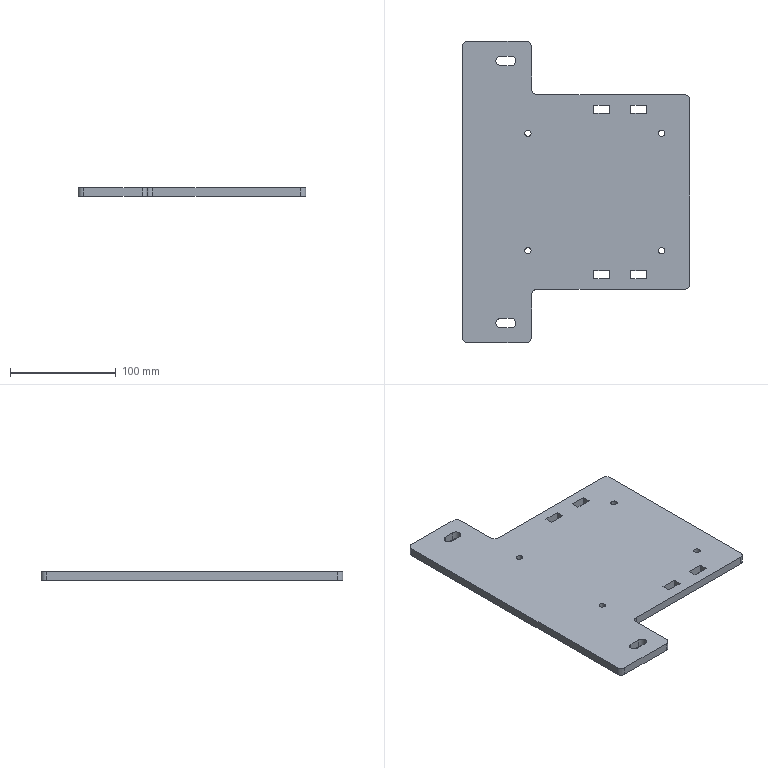Part | 1 solid | 52 faces | box 215 x 285 x 7.8 mm | volume 353300 mm3 | plane 30 | cylinder 22 | commonest cylinder face diameters 6 x8 10 x8 9 x6